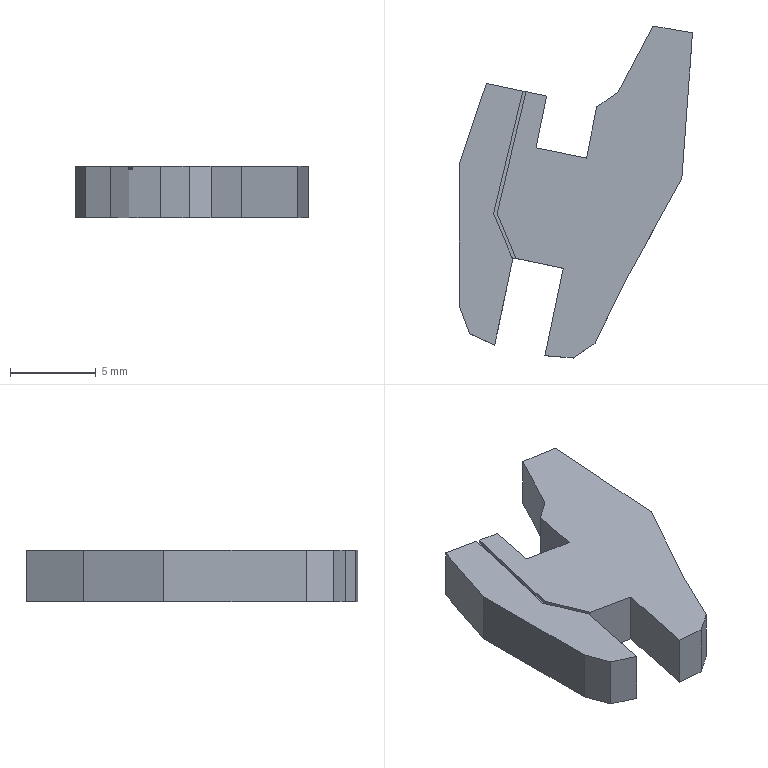Part | SolidWorks | features BaseBody 1 | 1 solid | 27 faces | box 13.603 x 19.375 x 3 mm | volume 451.595 mm3 | plane 15 | spline 12
STEP:
#1=CARTESIAN_POINT('',(66.198,112.5,1.3));
#2=VERTEX_POINT('',#1);
#3=CARTESIAN_POINT('',(66.394,112.459,1.3));
#4=VERTEX_POINT('',#3);
#5=CARTESIAN_POINT('',(66.198,112.5,1.3));
#6=CARTESIAN_POINT('',(66.263,112.486,1.3));
#7=CARTESIAN_POINT('',(66.329,112.473,1.3));
#8=CARTESIAN_POINT('',(66.394,112.459,1.3));
#9=B_SPLINE_CURVE_WITH_KNOTS('',3,(#5,#6,#7,#8),.UNSPECIFIED.,.F.,.F.,(4,4),(0.4488,0.4503),.UNSPECIFIED.);
#10=EDGE_CURVE('',#2,#4,#9,.T.);
#11=ORIENTED_EDGE('',*,*,#10,.F.);
#12=CARTESIAN_POINT('',(64.493,105.356,1.3));
#13=VERTEX_POINT('',#12);
#14=CARTESIAN_POINT('',(66.589,114.138,1.3));
#15=DIRECTION('',(-0.2321,-0.9727,0.));
#16=VECTOR('',#15,1000.);
#17=LINE('',#14,#16);
#18=EDGE_CURVE('',#2,#13,#17,.T.);
#19=ORIENTED_EDGE('',*,*,#18,.T.);
#20=CARTESIAN_POINT('',(65.611,102.69,1.3));
#21=VERTEX_POINT('',#20);
#22=CARTESIAN_POINT('',(64.493,105.356,1.3));
#23=DIRECTION('',(0.3866,-0.9222,0.));
#24=VECTOR('',#23,1000.);
#25=LINE('',#22,#24);
#26=EDGE_CURVE('',#13,#21,#25,.T.);
#27=ORIENTED_EDGE('',*,*,#26,.T.);
#28=CARTESIAN_POINT('',(65.627,102.768,1.3));
#29=VERTEX_POINT('',#28);
#30=CARTESIAN_POINT('',(42.225,-8.853,1.3));
#31=DIRECTION('',(0.2052,0.9787,0.));
#32=VECTOR('',#31,1000.);
#33=LINE('',#30,#32);
#34=EDGE_CURVE('',#21,#29,#33,.T.);
#35=ORIENTED_EDGE('',*,*,#34,.T.);
#36=CARTESIAN_POINT('',(65.811,102.729,1.3));
#37=VERTEX_POINT('',#36);
#38=CARTESIAN_POINT('',(23.402,111.621,1.3));
#39=DIRECTION('',(-0.9787,0.2052,0.));
#40=VECTOR('',#39,1000.);
#41=LINE('',#38,#40);
#42=EDGE_CURVE('',#37,#29,#41,.T.);
#43=ORIENTED_EDGE('',*,*,#42,.F.);
#44=CARTESIAN_POINT('',(64.703,105.373,1.3));
#45=VERTEX_POINT('',#44);
#46=CARTESIAN_POINT('',(64.678,105.433,1.3));
#47=DIRECTION('',(0.3866,-0.9222,0.));
#48=VECTOR('',#47,1000.);
#49=LINE('',#46,#48);
#50=EDGE_CURVE('',#45,#37,#49,.T.);
#51=ORIENTED_EDGE('',*,*,#50,.F.);
#52=CARTESIAN_POINT('',(66.784,114.092,1.3));
#53=DIRECTION('',(-0.2321,-0.9727,0.));
#54=VECTOR('',#53,1000.);
#55=LINE('',#52,#54);
#56=EDGE_CURVE('',#4,#45,#55,.T.);
#57=ORIENTED_EDGE('',*,*,#56,.F.);
#58=EDGE_LOOP('',(#11,#19,#27,#35,#43,#51,#57));
#59=FACE_OUTER_BOUND('',#58,.T.);
#60=CARTESIAN_POINT('',(0.,0.,1.3));
#61=DIRECTION('',(0.,0.,-1.));
#62=DIRECTION('',(0.,-1.,0.));
#63=AXIS2_PLACEMENT_3D('',#60,#61,#62);
#64=PLANE('',#63);
#65=ADVANCED_FACE('',(#59),#64,.F.);
#66=ORIENTED_EDGE('',*,*,#18,.F.);
#67=CARTESIAN_POINT('',(66.198,112.5,1.5));
#68=VERTEX_POINT('',#67);
#69=CARTESIAN_POINT('',(66.198,112.5,1.5));
#70=DIRECTION('',(0.,0.,1.));
#71=VECTOR('',#70,1000.);
#72=LINE('',#69,#71);
#73=EDGE_CURVE('',#2,#68,#72,.T.);
#74=ORIENTED_EDGE('',*,*,#73,.T.);
#75=CARTESIAN_POINT('',(64.493,105.356,1.5));
#76=VERTEX_POINT('',#75);
#77=CARTESIAN_POINT('',(37.228,-8.885,1.5));
#78=DIRECTION('',(-0.2321,-0.9727,0.));
#79=VECTOR('',#78,1000.);
#80=LINE('',#77,#79);
#81=EDGE_CURVE('',#68,#76,#80,.T.);
#82=ORIENTED_EDGE('',*,*,#81,.T.);
#83=CARTESIAN_POINT('',(64.493,105.356,1.3));
#84=DIRECTION('',(0.,0.,1.));
#85=VECTOR('',#84,1000.);
#86=LINE('',#83,#85);
#87=EDGE_CURVE('',#13,#76,#86,.T.);
#88=ORIENTED_EDGE('',*,*,#87,.F.);
#89=EDGE_LOOP('',(#66,#74,#82,#88));
#90=FACE_OUTER_BOUND('',#89,.T.);
#91=CARTESIAN_POINT('',(66.589,114.138,1.3));
#92=DIRECTION('',(0.9727,-0.2321,0.));
#93=DIRECTION('',(0.,0.,-1.));
#94=AXIS2_PLACEMENT_3D('',#91,#92,#93);
#95=PLANE('',#94);
#96=ADVANCED_FACE('',(#90),#95,.T.);
#97=CARTESIAN_POINT('',(66.394,112.459,1.5));
#98=VERTEX_POINT('',#97);
#99=CARTESIAN_POINT('',(66.394,112.459,1.5));
#100=DIRECTION('',(0.,0.,1.));
#101=VECTOR('',#100,1000.);
#102=LINE('',#99,#101);
#103=EDGE_CURVE('',#4,#98,#102,.T.);
#104=ORIENTED_EDGE('',*,*,#103,.F.);
#105=ORIENTED_EDGE('',*,*,#56,.T.);
#106=CARTESIAN_POINT('',(64.703,105.373,1.5));
#107=VERTEX_POINT('',#106);
#108=CARTESIAN_POINT('',(64.703,105.373,1.3));
#109=DIRECTION('',(0.,0.,1.));
#110=VECTOR('',#109,1000.);
#111=LINE('',#108,#110);
#112=EDGE_CURVE('',#45,#107,#111,.T.);
#113=ORIENTED_EDGE('',*,*,#112,.T.);
#114=CARTESIAN_POINT('',(37.423,-8.931,1.5));
#115=DIRECTION('',(-0.2321,-0.9727,0.));
#116=VECTOR('',#115,1000.);
#117=LINE('',#114,#116);
#118=EDGE_CURVE('',#98,#107,#117,.T.);
#119=ORIENTED_EDGE('',*,*,#118,.F.);
#120=EDGE_LOOP('',(#104,#105,#113,#119));
#121=FACE_OUTER_BOUND('',#120,.T.);
#122=CARTESIAN_POINT('',(66.784,114.092,1.3));
#123=DIRECTION('',(0.9727,-0.2321,0.));
#124=DIRECTION('',(0.,0.,-1.));
#125=AXIS2_PLACEMENT_3D('',#122,#123,#124);
#126=PLANE('',#125);
#127=ADVANCED_FACE('',(#121),#126,.F.);
#128=CARTESIAN_POINT('',(65.811,102.729,1.5));
#129=VERTEX_POINT('',#128);
#130=CARTESIAN_POINT('',(65.811,102.729,1.5));
#131=DIRECTION('',(0.,0.,-1.));
#132=VECTOR('',#131,1000.);
#133=LINE('',#130,#132);
#134=EDGE_CURVE('',#129,#37,#133,.T.);
#135=ORIENTED_EDGE('',*,*,#134,.F.);
#136=CARTESIAN_POINT('',(64.678,105.433,1.5));
#137=DIRECTION('',(0.3866,-0.9222,0.));
#138=VECTOR('',#137,1000.);
#139=LINE('',#136,#138);
#140=EDGE_CURVE('',#107,#129,#139,.T.);
#141=ORIENTED_EDGE('',*,*,#140,.F.);
#142=ORIENTED_EDGE('',*,*,#112,.F.);
#143=ORIENTED_EDGE('',*,*,#50,.T.);
#144=EDGE_LOOP('',(#135,#141,#142,#143));
#145=FACE_OUTER_BOUND('',#144,.T.);
#146=CARTESIAN_POINT('',(64.678,105.433,1.3));
#147=DIRECTION('',(0.9222,0.3866,0.));
#148=DIRECTION('',(0.,0.,-1.));
#149=AXIS2_PLACEMENT_3D('',#146,#147,#148);
#150=PLANE('',#149);
#151=ADVANCED_FACE('',(#145),#150,.F.);
#152=CARTESIAN_POINT('',(65.611,102.69,1.5));
#153=VERTEX_POINT('',#152);
#154=CARTESIAN_POINT('',(65.611,102.69,1.5));
#155=DIRECTION('',(0.,0.,1.));
#156=VECTOR('',#155,1000.);
#157=LINE('',#154,#156);
#158=EDGE_CURVE('',#21,#153,#157,.T.);
#159=ORIENTED_EDGE('',*,*,#158,.F.);
#160=ORIENTED_EDGE('',*,*,#26,.F.);
#161=ORIENTED_EDGE('',*,*,#87,.T.);
#162=CARTESIAN_POINT('',(64.493,105.356,1.5));
#163=DIRECTION('',(0.3866,-0.9222,0.));
#164=VECTOR('',#163,1000.);
#165=LINE('',#162,#164);
#166=EDGE_CURVE('',#76,#153,#165,.T.);
#167=ORIENTED_EDGE('',*,*,#166,.T.);
#168=EDGE_LOOP('',(#159,#160,#161,#167));
#169=FACE_OUTER_BOUND('',#168,.T.);
#170=CARTESIAN_POINT('',(64.493,105.356,1.3));
#171=DIRECTION('',(0.9222,0.3866,0.));
#172=DIRECTION('',(0.,0.,-1.));
#173=AXIS2_PLACEMENT_3D('',#170,#171,#172);
#174=PLANE('',#173);
#175=ADVANCED_FACE('',(#169),#174,.T.);
#176=CARTESIAN_POINT('',(64.074,112.946,-1.5));
#177=VERTEX_POINT('',#176);
#178=CARTESIAN_POINT('',(62.506,108.263,-1.5));
#179=VERTEX_POINT('',#178);
#180=CARTESIAN_POINT('',(64.074,112.946,-1.5));
#181=CARTESIAN_POINT('',(63.551,111.385,-1.5));
#182=CARTESIAN_POINT('',(63.029,109.824,-1.5));
#183=CARTESIAN_POINT('',(62.506,108.263,-1.5));
#184=B_SPLINE_CURVE_WITH_KNOTS('',3,(#180,#181,#182,#183),.UNSPECIFIED.,.F.,.F.,(4,4),(0.4595,0.4865),.UNSPECIFIED.);
#185=EDGE_CURVE('',#177,#179,#184,.T.);
#186=ORIENTED_EDGE('',*,*,#185,.F.);
#187=CARTESIAN_POINT('',(67.59,112.208,-1.5));
#188=VERTEX_POINT('',#187);
#189=CARTESIAN_POINT('',(67.59,112.208,-1.5));
#190=CARTESIAN_POINT('',(66.416,112.454,-1.5));
#191=CARTESIAN_POINT('',(65.247,112.7,-1.5));
#192=CARTESIAN_POINT('',(64.074,112.946,-1.5));
#193=B_SPLINE_CURVE_WITH_KNOTS('',3,(#189,#190,#191,#192),.UNSPECIFIED.,.F.,.F.,(4,4),(0.4324,0.4595),.UNSPECIFIED.);
#194=EDGE_CURVE('',#188,#177,#193,.T.);
#195=ORIENTED_EDGE('',*,*,#194,.F.);
#196=CARTESIAN_POINT('',(66.974,109.185,-1.5));
#197=VERTEX_POINT('',#196);
#198=CARTESIAN_POINT('',(42.966,-8.747,-1.5));
#199=DIRECTION('',(-0.1995,-0.9799,0.));
#200=VECTOR('',#199,1000.);
#201=LINE('',#198,#200);
#202=EDGE_CURVE('',#188,#197,#201,.T.);
#203=ORIENTED_EDGE('',*,*,#202,.T.);
#204=CARTESIAN_POINT('',(69.914,108.586,-1.5));
#205=VERTEX_POINT('',#204);
#206=CARTESIAN_POINT('',(24.008,117.932,-1.5));
#207=DIRECTION('',(0.9799,-0.1995,0.));
#208=VECTOR('',#207,1000.);
#209=LINE('',#206,#208);
#210=EDGE_CURVE('',#197,#205,#209,.T.);
#211=ORIENTED_EDGE('',*,*,#210,.T.);
#212=CARTESIAN_POINT('',(70.523,111.576,-1.5));
#213=VERTEX_POINT('',#212);
#214=CARTESIAN_POINT('',(45.905,-9.345,-1.5));
#215=DIRECTION('',(-0.1995,-0.9799,0.));
#216=VECTOR('',#215,1000.);
#217=LINE('',#214,#216);
#218=EDGE_CURVE('',#213,#205,#217,.T.);
#219=ORIENTED_EDGE('',*,*,#218,.F.);
#220=CARTESIAN_POINT('',(71.782,112.463,-1.5));
#221=VERTEX_POINT('',#220);
#222=CARTESIAN_POINT('',(71.782,112.463,-1.5));
#223=CARTESIAN_POINT('',(71.368,112.172,-1.5));
#224=CARTESIAN_POINT('',(70.946,111.878,-1.5));
#225=CARTESIAN_POINT('',(70.529,111.581,-1.5));
#226=CARTESIAN_POINT('',(70.523,111.576,-1.5));
#227=B_SPLINE_CURVE_WITH_KNOTS('',3,(#222,#223,#224,#225,#226),.UNSPECIFIED.,.F.,.F.,(4,1,4),(0.3243,0.3514,0.3518),.UNSPECIFIED.);
#228=EDGE_CURVE('',#221,#213,#227,.T.);
#229=ORIENTED_EDGE('',*,*,#228,.F.);
#230=CARTESIAN_POINT('',(73.791,116.299,-1.5));
#231=VERTEX_POINT('',#230);
#232=CARTESIAN_POINT('',(73.791,116.299,-1.5));
#233=CARTESIAN_POINT('',(73.122,115.02,-1.5));
#234=CARTESIAN_POINT('',(72.451,113.741,-1.5));
#235=CARTESIAN_POINT('',(71.782,112.463,-1.5));
#236=B_SPLINE_CURVE_WITH_KNOTS('',3,(#232,#233,#234,#235),.UNSPECIFIED.,.F.,.F.,(4,4),(0.2973,0.3243),.UNSPECIFIED.);
#237=EDGE_CURVE('',#231,#221,#236,.T.);
#238=ORIENTED_EDGE('',*,*,#237,.F.);
#239=CARTESIAN_POINT('',(76.109,115.9,-1.5));
#240=VERTEX_POINT('',#239);
#241=CARTESIAN_POINT('',(76.109,115.9,-1.5));
#242=CARTESIAN_POINT('',(75.336,116.034,-1.5));
#243=CARTESIAN_POINT('',(74.563,116.165,-1.5));
#244=CARTESIAN_POINT('',(73.791,116.299,-1.5));
#245=B_SPLINE_CURVE_WITH_KNOTS('',3,(#241,#242,#243,#244),.UNSPECIFIED.,.F.,.F.,(4,4),(0.2703,0.2973),.UNSPECIFIED.);
#246=EDGE_CURVE('',#240,#231,#245,.T.);
#247=ORIENTED_EDGE('',*,*,#246,.F.);
#248=CARTESIAN_POINT('',(75.486,107.399,-1.5));
#249=VERTEX_POINT('',#248);
#250=CARTESIAN_POINT('',(75.486,107.399,-1.5));
#251=CARTESIAN_POINT('',(75.695,110.235,-1.5));
#252=CARTESIAN_POINT('',(75.9,113.068,-1.5));
#253=CARTESIAN_POINT('',(76.109,115.9,-1.5));
#254=B_SPLINE_CURVE_WITH_KNOTS('',3,(#250,#251,#252,#253),.UNSPECIFIED.,.F.,.F.,(4,4),(0.2432,0.2703),.UNSPECIFIED.);
#255=EDGE_CURVE('',#249,#240,#254,.T.);
#256=ORIENTED_EDGE('',*,*,#255,.F.);
#257=CARTESIAN_POINT('',(72.174,101.392,-1.5));
#258=VERTEX_POINT('',#257);
#259=CARTESIAN_POINT('',(72.174,101.392,-1.5));
#260=CARTESIAN_POINT('',(73.277,103.395,-1.5));
#261=CARTESIAN_POINT('',(74.383,105.398,-1.5));
#262=CARTESIAN_POINT('',(75.486,107.399,-1.5));
#263=B_SPLINE_CURVE_WITH_KNOTS('',3,(#259,#260,#261,#262),.UNSPECIFIED.,.F.,.F.,(4,4),(0.2162,0.2432),.UNSPECIFIED.);
#264=EDGE_CURVE('',#258,#249,#263,.T.);
#265=ORIENTED_EDGE('',*,*,#264,.F.);
#266=CARTESIAN_POINT('',(70.417,97.774,-1.5));
#267=VERTEX_POINT('',#266);
#268=CARTESIAN_POINT('',(70.417,97.774,-1.5));
#269=CARTESIAN_POINT('',(71.002,98.978,-1.5));
#270=CARTESIAN_POINT('',(71.586,100.184,-1.5));
#271=CARTESIAN_POINT('',(72.174,101.392,-1.5));
#272=B_SPLINE_CURVE_WITH_KNOTS('',3,(#268,#269,#270,#271),.UNSPECIFIED.,.F.,.F.,(4,4),(0.1892,0.2162),.UNSPECIFIED.);
#273=EDGE_CURVE('',#267,#258,#272,.T.);
#274=ORIENTED_EDGE('',*,*,#273,.F.);
#275=CARTESIAN_POINT('',(69.133,96.923,-1.5));
#276=VERTEX_POINT('',#275);
#277=CARTESIAN_POINT('',(69.133,96.923,-1.5));
#278=CARTESIAN_POINT('',(69.561,97.206,-1.5));
#279=CARTESIAN_POINT('',(69.989,97.49,-1.5));
#280=CARTESIAN_POINT('',(70.417,97.774,-1.5));
#281=B_SPLINE_CURVE_WITH_KNOTS('',3,(#277,#278,#279,#280),.UNSPECIFIED.,.F.,.F.,(4,4),(0.1622,0.1892),.UNSPECIFIED.);
#282=EDGE_CURVE('',#276,#267,#281,.T.);
#283=ORIENTED_EDGE('',*,*,#282,.F.);
#284=CARTESIAN_POINT('',(67.494,97.055,-1.5));
#285=VERTEX_POINT('',#284);
#286=CARTESIAN_POINT('',(67.494,97.055,-1.5));
#287=CARTESIAN_POINT('',(68.041,97.01,-1.5));
#288=CARTESIAN_POINT('',(68.588,96.967,-1.5));
#289=CARTESIAN_POINT('',(69.133,96.923,-1.5));
#290=B_SPLINE_CURVE_WITH_KNOTS('',3,(#286,#287,#288,#289),.UNSPECIFIED.,.F.,.F.,(4,4),(0.1351,0.1622),.UNSPECIFIED.);
#291=EDGE_CURVE('',#285,#276,#290,.T.);
#292=ORIENTED_EDGE('',*,*,#291,.F.);
#293=CARTESIAN_POINT('',(68.563,102.152,-1.5));
#294=VERTEX_POINT('',#293);
#295=CARTESIAN_POINT('',(45.161,-9.468,-1.5));
#296=DIRECTION('',(-0.2052,-0.9787,0.));
#297=VECTOR('',#296,1000.);
#298=LINE('',#295,#297);
#299=EDGE_CURVE('',#294,#285,#298,.T.);
#300=ORIENTED_EDGE('',*,*,#299,.F.);
#301=CARTESIAN_POINT('',(65.627,102.768,-1.5));
#302=VERTEX_POINT('',#301);
#303=CARTESIAN_POINT('',(23.402,111.621,-1.5));
#304=DIRECTION('',(0.9787,-0.2052,0.));
#305=VECTOR('',#304,1000.);
#306=LINE('',#303,#305);
#307=EDGE_CURVE('',#302,#294,#306,.T.);
#308=ORIENTED_EDGE('',*,*,#307,.F.);
#309=CARTESIAN_POINT('',(64.558,97.671,-1.5));
#310=VERTEX_POINT('',#309);
#311=CARTESIAN_POINT('',(42.225,-8.853,-1.5));
#312=DIRECTION('',(-0.2052,-0.9787,0.));
#313=VECTOR('',#312,1000.);
#314=LINE('',#311,#313);
#315=EDGE_CURVE('',#302,#310,#314,.T.);
#316=ORIENTED_EDGE('',*,*,#315,.T.);
#317=CARTESIAN_POINT('',(63.093,98.343,-1.5));
#318=VERTEX_POINT('',#317);
#319=CARTESIAN_POINT('',(63.093,98.343,-1.5));
#320=CARTESIAN_POINT('',(63.582,98.12,-1.5));
#321=CARTESIAN_POINT('',(64.069,97.895,-1.5));
#322=CARTESIAN_POINT('',(64.558,97.671,-1.5));
#323=B_SPLINE_CURVE_WITH_KNOTS('',3,(#319,#320,#321,#322),.UNSPECIFIED.,.F.,.F.,(4,4),(0.02703,0.05397),.UNSPECIFIED.);
#324=EDGE_CURVE('',#318,#310,#323,.T.);
#325=ORIENTED_EDGE('',*,*,#324,.F.);
#326=CARTESIAN_POINT('',(62.506,99.936,-1.5));
#327=VERTEX_POINT('',#326);
#328=CARTESIAN_POINT('',(62.506,99.936,-1.5));
#329=CARTESIAN_POINT('',(62.702,99.405,-1.5));
#330=CARTESIAN_POINT('',(62.897,98.875,-1.5));
#331=CARTESIAN_POINT('',(63.093,98.343,-1.5));
#332=B_SPLINE_CURVE_WITH_KNOTS('',3,(#328,#329,#330,#331),.UNSPECIFIED.,.F.,.F.,(4,4),(0.,0.02703),.UNSPECIFIED.);
#333=EDGE_CURVE('',#327,#318,#332,.T.);
#334=ORIENTED_EDGE('',*,*,#333,.F.);
#335=CARTESIAN_POINT('',(62.506,0.,-1.5));
#336=DIRECTION('',(0.,-1.,0.));
#337=VECTOR('',#336,1000.);
#338=LINE('',#335,#337);
#339=EDGE_CURVE('',#179,#327,#338,.T.);
#340=ORIENTED_EDGE('',*,*,#339,.F.);
#341=EDGE_LOOP('',(#186,#195,#203,#211,#219,#229,#238,#247,#256,#265,#274,#283,#292,#300,#308,#316,#325,#334,#340));
#342=FACE_OUTER_BOUND('',#341,.T.);
#343=CARTESIAN_POINT('',(0.,0.,-1.5));
#344=DIRECTION('',(0.,0.,1.));
#345=DIRECTION('',(1.,0.,0.));
#346=AXIS2_PLACEMENT_3D('',#343,#344,#345);
#347=PLANE('',#346);
#348=ADVANCED_FACE('',(#342),#347,.F.);
#349=ORIENTED_EDGE('',*,*,#140,.T.);
#350=CARTESIAN_POINT('',(68.563,102.152,1.5));
#351=VERTEX_POINT('',#350);
#352=CARTESIAN_POINT('',(23.402,111.621,1.5));
#353=DIRECTION('',(0.9787,-0.2052,0.));
#354=VECTOR('',#353,1000.);
#355=LINE('',#352,#354);
#356=EDGE_CURVE('',#129,#351,#355,.T.);
#357=ORIENTED_EDGE('',*,*,#356,.T.);
#358=CARTESIAN_POINT('',(67.494,97.055,1.5));
#359=VERTEX_POINT('',#358);
#360=CARTESIAN_POINT('',(45.161,-9.468,1.5));
#361=DIRECTION('',(-0.2052,-0.9787,0.));
#362=VECTOR('',#361,1000.);
#363=LINE('',#360,#362);
#364=EDGE_CURVE('',#351,#359,#363,.T.);
#365=ORIENTED_EDGE('',*,*,#364,.T.);
#366=CARTESIAN_POINT('',(69.133,96.923,1.5));
#367=VERTEX_POINT('',#366);
#368=CARTESIAN_POINT('',(67.494,97.055,1.5));
#369=CARTESIAN_POINT('',(68.041,97.01,1.5));
#370=CARTESIAN_POINT('',(68.588,96.967,1.5));
#371=CARTESIAN_POINT('',(69.133,96.923,1.5));
#372=B_SPLINE_CURVE_WITH_KNOTS('',3,(#368,#369,#370,#371),.UNSPECIFIED.,.F.,.F.,(4,4),(0.1351,0.1622),.UNSPECIFIED.);
#373=EDGE_CURVE('',#359,#367,#372,.T.);
#374=ORIENTED_EDGE('',*,*,#373,.T.);
#375=CARTESIAN_POINT('',(70.417,97.774,1.5));
#376=VERTEX_POINT('',#375);
#377=CARTESIAN_POINT('',(69.133,96.923,1.5));
#378=CARTESIAN_POINT('',(69.561,97.206,1.5));
#379=CARTESIAN_POINT('',(69.989,97.49,1.5));
#380=CARTESIAN_POINT('',(70.417,97.774,1.5));
#381=B_SPLINE_CURVE_WITH_KNOTS('',3,(#377,#378,#379,#380),.UNSPECIFIED.,.F.,.F.,(4,4),(0.1622,0.1892),.UNSPECIFIED.);
#382=EDGE_CURVE('',#367,#376,#381,.T.);
#383=ORIENTED_EDGE('',*,*,#382,.T.);
#384=CARTESIAN_POINT('',(72.174,101.392,1.5));
#385=VERTEX_POINT('',#384);
#386=CARTESIAN_POINT('',(70.417,97.774,1.5));
#387=CARTESIAN_POINT('',(71.002,98.978,1.5));
#388=CARTESIAN_POINT('',(71.586,100.184,1.5));
#389=CARTESIAN_POINT('',(72.174,101.392,1.5));
#390=B_SPLINE_CURVE_WITH_KNOTS('',3,(#386,#387,#388,#389),.UNSPECIFIED.,.F.,.F.,(4,4),(0.1892,0.2162),.UNSPECIFIED.);
#391=EDGE_CURVE('',#376,#385,#390,.T.);
#392=ORIENTED_EDGE('',*,*,#391,.T.);
#393=CARTESIAN_POINT('',(75.486,107.399,1.5));
#394=VERTEX_POINT('',#393);
#395=CARTESIAN_POINT('',(72.174,101.392,1.5));
#396=CARTESIAN_POINT('',(73.277,103.395,1.5));
#397=CARTESIAN_POINT('',(74.383,105.398,1.5));
#398=CARTESIAN_POINT('',(75.486,107.399,1.5));
#399=B_SPLINE_CURVE_WITH_KNOTS('',3,(#395,#396,#397,#398),.UNSPECIFIED.,.F.,.F.,(4,4),(0.2162,0.2432),.UNSPECIFIED.);
#400=EDGE_CURVE('',#385,#394,#399,.T.);
#401=ORIENTED_EDGE('',*,*,#400,.T.);
#402=CARTESIAN_POINT('',(76.109,115.9,1.5));
#403=VERTEX_POINT('',#402);
#404=CARTESIAN_POINT('',(75.486,107.399,1.5));
#405=CARTESIAN_POINT('',(75.695,110.235,1.5));
#406=CARTESIAN_POINT('',(75.9,113.068,1.5));
#407=CARTESIAN_POINT('',(76.109,115.9,1.5));
#408=B_SPLINE_CURVE_WITH_KNOTS('',3,(#404,#405,#406,#407),.UNSPECIFIED.,.F.,.F.,(4,4),(0.2432,0.2703),.UNSPECIFIED.);
#409=EDGE_CURVE('',#394,#403,#408,.T.);
#410=ORIENTED_EDGE('',*,*,#409,.T.);
#411=CARTESIAN_POINT('',(73.791,116.299,1.5));
#412=VERTEX_POINT('',#411);
#413=CARTESIAN_POINT('',(76.109,115.9,1.5));
#414=CARTESIAN_POINT('',(75.336,116.034,1.5));
#415=CARTESIAN_POINT('',(74.563,116.165,1.5));
#416=CARTESIAN_POINT('',(73.791,116.299,1.5));
#417=B_SPLINE_CURVE_WITH_KNOTS('',3,(#413,#414,#415,#416),.UNSPECIFIED.,.F.,.F.,(4,4),(0.2703,0.2973),.UNSPECIFIED.);
#418=EDGE_CURVE('',#403,#412,#417,.T.);
#419=ORIENTED_EDGE('',*,*,#418,.T.);
#420=CARTESIAN_POINT('',(71.782,112.463,1.5));
#421=VERTEX_POINT('',#420);
#422=CARTESIAN_POINT('',(73.791,116.299,1.5));
#423=CARTESIAN_POINT('',(73.122,115.02,1.5));
#424=CARTESIAN_POINT('',(72.451,113.741,1.5));
#425=CARTESIAN_POINT('',(71.782,112.463,1.5));
#426=B_SPLINE_CURVE_WITH_KNOTS('',3,(#422,#423,#424,#425),.UNSPECIFIED.,.F.,.F.,(4,4),(0.2973,0.3243),.UNSPECIFIED.);
#427=EDGE_CURVE('',#412,#421,#426,.T.);
#428=ORIENTED_EDGE('',*,*,#427,.T.);
#429=CARTESIAN_POINT('',(70.523,111.576,1.5));
#430=VERTEX_POINT('',#429);
#431=CARTESIAN_POINT('',(71.782,112.463,1.5));
#432=CARTESIAN_POINT('',(71.368,112.172,1.5));
#433=CARTESIAN_POINT('',(70.946,111.878,1.5));
#434=CARTESIAN_POINT('',(70.529,111.581,1.5));
#435=CARTESIAN_POINT('',(70.523,111.576,1.5));
#436=B_SPLINE_CURVE_WITH_KNOTS('',3,(#431,#432,#433,#434,#435),.UNSPECIFIED.,.F.,.F.,(4,1,4),(0.3243,0.3514,0.3518),.UNSPECIFIED.);
#437=EDGE_CURVE('',#421,#430,#436,.T.);
#438=ORIENTED_EDGE('',*,*,#437,.T.);
#439=CARTESIAN_POINT('',(69.914,108.586,1.5));
#440=VERTEX_POINT('',#439);
#441=CARTESIAN_POINT('',(45.905,-9.345,1.5));
#442=DIRECTION('',(-0.1995,-0.9799,0.));
#443=VECTOR('',#442,1000.);
#444=LINE('',#441,#443);
#445=EDGE_CURVE('',#430,#440,#444,.T.);
#446=ORIENTED_EDGE('',*,*,#445,.T.);
#447=CARTESIAN_POINT('',(66.974,109.185,1.5));
#448=VERTEX_POINT('',#447);
#449=CARTESIAN_POINT('',(24.008,117.932,1.5));
#450=DIRECTION('',(0.9799,-0.1995,0.));
#451=VECTOR('',#450,1000.);
#452=LINE('',#449,#451);
#453=EDGE_CURVE('',#448,#440,#452,.T.);
#454=ORIENTED_EDGE('',*,*,#453,.F.);
#455=CARTESIAN_POINT('',(67.59,112.208,1.5));
#456=VERTEX_POINT('',#455);
#457=CARTESIAN_POINT('',(42.966,-8.747,1.5));
#458=DIRECTION('',(-0.1995,-0.9799,0.));
#459=VECTOR('',#458,1000.);
#460=LINE('',#457,#459);
#461=EDGE_CURVE('',#456,#448,#460,.T.);
#462=ORIENTED_EDGE('',*,*,#461,.F.);
#463=CARTESIAN_POINT('',(67.59,112.208,1.5));
#464=CARTESIAN_POINT('',(67.191,112.292,1.5));
#465=CARTESIAN_POINT('',(66.792,112.375,1.5));
#466=CARTESIAN_POINT('',(66.394,112.459,1.5));
#467=B_SPLINE_CURVE_WITH_KNOTS('',3,(#463,#464,#465,#466),.UNSPECIFIED.,.F.,.F.,(4,4),(0.4324,0.4416),.UNSPECIFIED.);
#468=EDGE_CURVE('',#456,#98,#467,.T.);
#469=ORIENTED_EDGE('',*,*,#468,.T.);
#470=ORIENTED_EDGE('',*,*,#118,.T.);
#471=EDGE_LOOP('',(#349,#357,#365,#374,#383,#392,#401,#410,#419,#428,#438,#446,#454,#462,#469,#470));
#472=FACE_OUTER_BOUND('',#471,.T.);
#473=CARTESIAN_POINT('',(0.,0.,1.5));
#474=DIRECTION('',(0.,0.,1.));
#475=DIRECTION('',(1.,0.,0.));
#476=AXIS2_PLACEMENT_3D('',#473,#474,#475);
#477=PLANE('',#476);
#478=ADVANCED_FACE('',(#472),#477,.T.);
#479=ORIENTED_EDGE('',*,*,#339,.T.);
#480=CARTESIAN_POINT('',(62.506,99.936,1.5));
#481=VERTEX_POINT('',#480);
#482=CARTESIAN_POINT('',(62.506,99.936,1.5));
#483=DIRECTION('',(0.,0.,-1.));
#484=VECTOR('',#483,1000.);
#485=LINE('',#482,#484);
#486=EDGE_CURVE('',#481,#327,#485,.T.);
#487=ORIENTED_EDGE('',*,*,#486,.F.);
#488=CARTESIAN_POINT('',(62.506,108.263,1.5));
#489=VERTEX_POINT('',#488);
#490=CARTESIAN_POINT('',(62.506,0.,1.5));
#491=DIRECTION('',(0.,-1.,0.));
#492=VECTOR('',#491,1000.);
#493=LINE('',#490,#492);
#494=EDGE_CURVE('',#489,#481,#493,.T.);
#495=ORIENTED_EDGE('',*,*,#494,.F.);
#496=CARTESIAN_POINT('',(62.506,108.263,1.5));
#497=DIRECTION('',(0.,0.,-1.));
#498=VECTOR('',#497,1000.);
#499=LINE('',#496,#498);
#500=EDGE_CURVE('',#489,#179,#499,.T.);
#501=ORIENTED_EDGE('',*,*,#500,.T.);
#502=EDGE_LOOP('',(#479,#487,#495,#501));
#503=FACE_OUTER_BOUND('',#502,.T.);
#504=CARTESIAN_POINT('',(62.506,0.,1.5));
#505=DIRECTION('',(-1.,0.,0.));
#506=DIRECTION('',(0.,0.,1.));
#507=AXIS2_PLACEMENT_3D('',#504,#505,#506);
#508=PLANE('',#507);
#509=ADVANCED_FACE('',(#503),#508,.T.);
#510=ORIENTED_EDGE('',*,*,#333,.T.);
#511=CARTESIAN_POINT('',(63.093,98.343,1.5));
#512=VERTEX_POINT('',#511);
#513=CARTESIAN_POINT('',(63.093,98.343,1.5));
#514=DIRECTION('',(0.,0.,-1.));
#515=VECTOR('',#514,1000.);
#516=LINE('',#513,#515);
#517=EDGE_CURVE('',#512,#318,#516,.T.);
#518=ORIENTED_EDGE('',*,*,#517,.F.);
#519=CARTESIAN_POINT('',(62.506,99.936,1.5));
#520=CARTESIAN_POINT('',(62.702,99.405,1.5));
#521=CARTESIAN_POINT('',(62.897,98.875,1.5));
#522=CARTESIAN_POINT('',(63.093,98.343,1.5));
#523=B_SPLINE_CURVE_WITH_KNOTS('',3,(#519,#520,#521,#522),.UNSPECIFIED.,.F.,.F.,(4,4),(0.,0.02703),.UNSPECIFIED.);
#524=EDGE_CURVE('',#481,#512,#523,.T.);
#525=ORIENTED_EDGE('',*,*,#524,.F.);
#526=ORIENTED_EDGE('',*,*,#486,.T.);
#527=EDGE_LOOP('',(#510,#518,#525,#526));
#528=FACE_OUTER_BOUND('',#527,.T.);
#529=CARTESIAN_POINT('',(63.093,98.343,1.5));
#530=CARTESIAN_POINT('',(63.093,98.343,-1.5));
#531=CARTESIAN_POINT('',(62.897,98.875,1.5));
#532=CARTESIAN_POINT('',(62.897,98.875,-1.5));
#533=CARTESIAN_POINT('',(62.702,99.405,1.5));
#534=CARTESIAN_POINT('',(62.702,99.405,-1.5));
#535=CARTESIAN_POINT('',(62.506,99.936,1.5));
#536=CARTESIAN_POINT('',(62.506,99.936,-1.5));
#537=B_SPLINE_SURFACE_WITH_KNOTS('',3,1,((#529,#530),(#531,#532),(#533,#534),(#535,#536)),.UNSPECIFIED.,.F.,.F.,.F.,(4,4),(2,2),(0.,0.02703),(0.,1.),.UNSPECIFIED.);
#538=ADVANCED_FACE('',(#528),#537,.T.);
#539=ORIENTED_EDGE('',*,*,#324,.T.);
#540=CARTESIAN_POINT('',(64.558,97.671,1.5));
#541=VERTEX_POINT('',#540);
#542=CARTESIAN_POINT('',(64.558,97.671,1.5));
#543=DIRECTION('',(0.,0.,-1.));
#544=VECTOR('',#543,1000.);
#545=LINE('',#542,#544);
#546=EDGE_CURVE('',#541,#310,#545,.T.);
#547=ORIENTED_EDGE('',*,*,#546,.F.);
#548=CARTESIAN_POINT('',(63.093,98.343,1.5));
#549=CARTESIAN_POINT('',(63.582,98.12,1.5));
#550=CARTESIAN_POINT('',(64.069,97.895,1.5));
#551=CARTESIAN_POINT('',(64.558,97.671,1.5));
#552=B_SPLINE_CURVE_WITH_KNOTS('',3,(#548,#549,#550,#551),.UNSPECIFIED.,.F.,.F.,(4,4),(0.02703,0.05397),.UNSPECIFIED.);
#553=EDGE_CURVE('',#512,#541,#552,.T.);
#554=ORIENTED_EDGE('',*,*,#553,.F.);
#555=ORIENTED_EDGE('',*,*,#517,.T.);
#556=EDGE_LOOP('',(#539,#547,#554,#555));
#557=FACE_OUTER_BOUND('',#556,.T.);
#558=CARTESIAN_POINT('',(64.558,97.671,1.5));
#559=CARTESIAN_POINT('',(64.558,97.671,-1.5));
#560=CARTESIAN_POINT('',(64.069,97.895,1.5));
#561=CARTESIAN_POINT('',(64.069,97.895,-1.5));
#562=CARTESIAN_POINT('',(63.582,98.12,1.5));
#563=CARTESIAN_POINT('',(63.582,98.12,-1.5));
#564=CARTESIAN_POINT('',(63.093,98.343,1.5));
#565=CARTESIAN_POINT('',(63.093,98.343,-1.5));
#566=B_SPLINE_SURFACE_WITH_KNOTS('',3,1,((#558,#559),(#560,#561),(#562,#563),(#564,#565)),.UNSPECIFIED.,.F.,.F.,.F.,(4,4),(2,2),(0.,0.02694),(0.,1.),.UNSPECIFIED.);
#567=ADVANCED_FACE('',(#557),#566,.T.);
#568=ORIENTED_EDGE('',*,*,#134,.T.);
#569=ORIENTED_EDGE('',*,*,#42,.T.);
#570=CARTESIAN_POINT('',(65.627,102.768,1.5));
#571=DIRECTION('',(0.,0.,-1.));
#572=VECTOR('',#571,1000.);
#573=LINE('',#570,#572);
#574=EDGE_CURVE('',#29,#302,#573,.T.);
#575=ORIENTED_EDGE('',*,*,#574,.T.);
#576=ORIENTED_EDGE('',*,*,#307,.T.);
#577=CARTESIAN_POINT('',(68.563,102.152,1.5));
#578=DIRECTION('',(0.,0.,-1.));
#579=VECTOR('',#578,1000.);
#580=LINE('',#577,#579);
#581=EDGE_CURVE('',#351,#294,#580,.T.);
#582=ORIENTED_EDGE('',*,*,#581,.F.);
#583=ORIENTED_EDGE('',*,*,#356,.F.);
#584=EDGE_LOOP('',(#568,#569,#575,#576,#582,#583));
#585=FACE_OUTER_BOUND('',#584,.T.);
#586=CARTESIAN_POINT('',(23.402,111.621,1.5));
#587=DIRECTION('',(-0.2052,-0.9787,0.));
#588=DIRECTION('',(-0.9787,0.2052,0.));
#589=AXIS2_PLACEMENT_3D('',#586,#587,#588);
#590=PLANE('',#589);
#591=ADVANCED_FACE('',(#585),#590,.T.);
#592=ORIENTED_EDGE('',*,*,#299,.T.);
#593=CARTESIAN_POINT('',(67.494,97.055,1.5));
#594=DIRECTION('',(0.,0.,-1.));
#595=VECTOR('',#594,1000.);
#596=LINE('',#593,#595);
#597=EDGE_CURVE('',#359,#285,#596,.T.);
#598=ORIENTED_EDGE('',*,*,#597,.F.);
#599=ORIENTED_EDGE('',*,*,#364,.F.);
#600=ORIENTED_EDGE('',*,*,#581,.T.);
#601=EDGE_LOOP('',(#592,#598,#599,#600));
#602=FACE_OUTER_BOUND('',#601,.T.);
#603=CARTESIAN_POINT('',(45.161,-9.468,1.5));
#604=DIRECTION('',(-0.9787,0.2052,0.));
#605=DIRECTION('',(0.,0.,1.));
#606=AXIS2_PLACEMENT_3D('',#603,#604,#605);
#607=PLANE('',#606);
#608=ADVANCED_FACE('',(#602),#607,.T.);
#609=ORIENTED_EDGE('',*,*,#291,.T.);
#610=CARTESIAN_POINT('',(69.133,96.923,1.5));
#611=DIRECTION('',(0.,0.,-1.));
#612=VECTOR('',#611,1000.);
#613=LINE('',#610,#612);
#614=EDGE_CURVE('',#367,#276,#613,.T.);
#615=ORIENTED_EDGE('',*,*,#614,.F.);
#616=ORIENTED_EDGE('',*,*,#373,.F.);
#617=ORIENTED_EDGE('',*,*,#597,.T.);
#618=EDGE_LOOP('',(#609,#615,#616,#617));
#619=FACE_OUTER_BOUND('',#618,.T.);
#620=CARTESIAN_POINT('',(69.133,96.923,1.5));
#621=CARTESIAN_POINT('',(69.133,96.923,-1.5));
#622=CARTESIAN_POINT('',(68.588,96.967,1.5));
#623=CARTESIAN_POINT('',(68.588,96.967,-1.5));
#624=CARTESIAN_POINT('',(68.041,97.01,1.5));
#625=CARTESIAN_POINT('',(68.041,97.01,-1.5));
#626=CARTESIAN_POINT('',(67.494,97.055,1.5));
#627=CARTESIAN_POINT('',(67.494,97.055,-1.5));
#628=B_SPLINE_SURFACE_WITH_KNOTS('',3,1,((#620,#621),(#622,#623),(#624,#625),(#626,#627)),.UNSPECIFIED.,.F.,.F.,.F.,(4,4),(2,2),(0.,0.02703),(0.,1.),.UNSPECIFIED.);
#629=ADVANCED_FACE('',(#619),#628,.T.);
#630=ORIENTED_EDGE('',*,*,#282,.T.);
#631=CARTESIAN_POINT('',(70.417,97.774,1.5));
#632=DIRECTION('',(0.,0.,-1.));
#633=VECTOR('',#632,1000.);
#634=LINE('',#631,#633);
#635=EDGE_CURVE('',#376,#267,#634,.T.);
#636=ORIENTED_EDGE('',*,*,#635,.F.);
#637=ORIENTED_EDGE('',*,*,#382,.F.);
#638=ORIENTED_EDGE('',*,*,#614,.T.);
#639=EDGE_LOOP('',(#630,#636,#637,#638));
#640=FACE_OUTER_BOUND('',#639,.T.);
#641=CARTESIAN_POINT('',(70.417,97.774,1.5));
#642=CARTESIAN_POINT('',(70.417,97.774,-1.5));
#643=CARTESIAN_POINT('',(69.989,97.49,1.5));
#644=CARTESIAN_POINT('',(69.989,97.49,-1.5));
#645=CARTESIAN_POINT('',(69.561,97.206,1.5));
#646=CARTESIAN_POINT('',(69.561,97.206,-1.5));
#647=CARTESIAN_POINT('',(69.133,96.923,1.5));
#648=CARTESIAN_POINT('',(69.133,96.923,-1.5));
#649=B_SPLINE_SURFACE_WITH_KNOTS('',3,1,((#641,#642),(#643,#644),(#645,#646),(#647,#648)),.UNSPECIFIED.,.F.,.F.,.F.,(4,4),(2,2),(0.,0.02703),(0.,1.),.UNSPECIFIED.);
#650=ADVANCED_FACE('',(#640),#649,.T.);
#651=ORIENTED_EDGE('',*,*,#273,.T.);
#652=CARTESIAN_POINT('',(72.174,101.392,1.5));
#653=DIRECTION('',(0.,0.,-1.));
#654=VECTOR('',#653,1000.);
#655=LINE('',#652,#654);
#656=EDGE_CURVE('',#385,#258,#655,.T.);
#657=ORIENTED_EDGE('',*,*,#656,.F.);
#658=ORIENTED_EDGE('',*,*,#391,.F.);
#659=ORIENTED_EDGE('',*,*,#635,.T.);
#660=EDGE_LOOP('',(#651,#657,#658,#659));
#661=FACE_OUTER_BOUND('',#660,.T.);
#662=CARTESIAN_POINT('',(72.174,101.392,1.5));
#663=CARTESIAN_POINT('',(72.174,101.392,-1.5));
#664=CARTESIAN_POINT('',(71.586,100.184,1.5));
#665=CARTESIAN_POINT('',(71.586,100.184,-1.5));
#666=CARTESIAN_POINT('',(71.002,98.978,1.5));
#667=CARTESIAN_POINT('',(71.002,98.978,-1.5));
#668=CARTESIAN_POINT('',(70.417,97.774,1.5));
#669=CARTESIAN_POINT('',(70.417,97.774,-1.5));
#670=B_SPLINE_SURFACE_WITH_KNOTS('',3,1,((#662,#663),(#664,#665),(#666,#667),(#668,#669)),.UNSPECIFIED.,.F.,.F.,.F.,(4,4),(2,2),(0.,0.02703),(0.,1.),.UNSPECIFIED.);
#671=ADVANCED_FACE('',(#661),#670,.T.);
#672=ORIENTED_EDGE('',*,*,#264,.T.);
#673=CARTESIAN_POINT('',(75.486,107.399,1.5));
#674=DIRECTION('',(0.,0.,-1.));
#675=VECTOR('',#674,1000.);
#676=LINE('',#673,#675);
#677=EDGE_CURVE('',#394,#249,#676,.T.);
#678=ORIENTED_EDGE('',*,*,#677,.F.);
#679=ORIENTED_EDGE('',*,*,#400,.F.);
#680=ORIENTED_EDGE('',*,*,#656,.T.);
#681=EDGE_LOOP('',(#672,#678,#679,#680));
#682=FACE_OUTER_BOUND('',#681,.T.);
#683=CARTESIAN_POINT('',(75.486,107.399,1.5));
#684=CARTESIAN_POINT('',(75.486,107.399,-1.5));
#685=CARTESIAN_POINT('',(74.383,105.398,1.5));
#686=CARTESIAN_POINT('',(74.383,105.398,-1.5));
#687=CARTESIAN_POINT('',(73.277,103.395,1.5));
#688=CARTESIAN_POINT('',(73.277,103.395,-1.5));
#689=CARTESIAN_POINT('',(72.174,101.392,1.5));
#690=CARTESIAN_POINT('',(72.174,101.392,-1.5));
#691=B_SPLINE_SURFACE_WITH_KNOTS('',3,1,((#683,#684),(#685,#686),(#687,#688),(#689,#690)),.UNSPECIFIED.,.F.,.F.,.F.,(4,4),(2,2),(0.,0.02703),(0.,1.),.UNSPECIFIED.);
#692=ADVANCED_FACE('',(#682),#691,.T.);
#693=ORIENTED_EDGE('',*,*,#255,.T.);
#694=CARTESIAN_POINT('',(76.109,115.9,1.5));
#695=DIRECTION('',(0.,0.,-1.));
#696=VECTOR('',#695,1000.);
#697=LINE('',#694,#696);
#698=EDGE_CURVE('',#403,#240,#697,.T.);
#699=ORIENTED_EDGE('',*,*,#698,.F.);
#700=ORIENTED_EDGE('',*,*,#409,.F.);
#701=ORIENTED_EDGE('',*,*,#677,.T.);
#702=EDGE_LOOP('',(#693,#699,#700,#701));
#703=FACE_OUTER_BOUND('',#702,.T.);
#704=CARTESIAN_POINT('',(76.109,115.9,1.5));
#705=CARTESIAN_POINT('',(76.109,115.9,-1.5));
#706=CARTESIAN_POINT('',(75.9,113.068,1.5));
#707=CARTESIAN_POINT('',(75.9,113.068,-1.5));
#708=CARTESIAN_POINT('',(75.695,110.235,1.5));
#709=CARTESIAN_POINT('',(75.695,110.235,-1.5));
#710=CARTESIAN_POINT('',(75.486,107.399,1.5));
#711=CARTESIAN_POINT('',(75.486,107.399,-1.5));
#712=B_SPLINE_SURFACE_WITH_KNOTS('',3,1,((#704,#705),(#706,#707),(#708,#709),(#710,#711)),.UNSPECIFIED.,.F.,.F.,.F.,(4,4),(2,2),(0.,0.02703),(0.,1.),.UNSPECIFIED.);
#713=ADVANCED_FACE('',(#703),#712,.T.);
#714=ORIENTED_EDGE('',*,*,#246,.T.);
#715=CARTESIAN_POINT('',(73.791,116.299,1.5));
#716=DIRECTION('',(0.,0.,-1.));
#717=VECTOR('',#716,1000.);
#718=LINE('',#715,#717);
#719=EDGE_CURVE('',#412,#231,#718,.T.);
#720=ORIENTED_EDGE('',*,*,#719,.F.);
#721=ORIENTED_EDGE('',*,*,#418,.F.);
#722=ORIENTED_EDGE('',*,*,#698,.T.);
#723=EDGE_LOOP('',(#714,#720,#721,#722));
#724=FACE_OUTER_BOUND('',#723,.T.);
#725=CARTESIAN_POINT('',(73.791,116.299,1.5));
#726=CARTESIAN_POINT('',(73.791,116.299,-1.5));
#727=CARTESIAN_POINT('',(74.563,116.165,1.5));
#728=CARTESIAN_POINT('',(74.563,116.165,-1.5));
#729=CARTESIAN_POINT('',(75.336,116.034,1.5));
#730=CARTESIAN_POINT('',(75.336,116.034,-1.5));
#731=CARTESIAN_POINT('',(76.109,115.9,1.5));
#732=CARTESIAN_POINT('',(76.109,115.9,-1.5));
#733=B_SPLINE_SURFACE_WITH_KNOTS('',3,1,((#725,#726),(#727,#728),(#729,#730),(#731,#732)),.UNSPECIFIED.,.F.,.F.,.F.,(4,4),(2,2),(0.,0.02703),(0.,1.),.UNSPECIFIED.);
#734=ADVANCED_FACE('',(#724),#733,.T.);
#735=ORIENTED_EDGE('',*,*,#237,.T.);
#736=CARTESIAN_POINT('',(71.782,112.463,1.5));
#737=DIRECTION('',(0.,0.,-1.));
#738=VECTOR('',#737,1000.);
#739=LINE('',#736,#738);
#740=EDGE_CURVE('',#421,#221,#739,.T.);
#741=ORIENTED_EDGE('',*,*,#740,.F.);
#742=ORIENTED_EDGE('',*,*,#427,.F.);
#743=ORIENTED_EDGE('',*,*,#719,.T.);
#744=EDGE_LOOP('',(#735,#741,#742,#743));
#745=FACE_OUTER_BOUND('',#744,.T.);
#746=CARTESIAN_POINT('',(71.782,112.463,1.5));
#747=CARTESIAN_POINT('',(71.782,112.463,-1.5));
#748=CARTESIAN_POINT('',(72.451,113.741,1.5));
#749=CARTESIAN_POINT('',(72.451,113.741,-1.5));
#750=CARTESIAN_POINT('',(73.122,115.02,1.5));
#751=CARTESIAN_POINT('',(73.122,115.02,-1.5));
#752=CARTESIAN_POINT('',(73.791,116.299,1.5));
#753=CARTESIAN_POINT('',(73.791,116.299,-1.5));
#754=B_SPLINE_SURFACE_WITH_KNOTS('',3,1,((#746,#747),(#748,#749),(#750,#751),(#752,#753)),.UNSPECIFIED.,.F.,.F.,.F.,(4,4),(2,2),(0.,0.02703),(0.,1.),.UNSPECIFIED.);
#755=ADVANCED_FACE('',(#745),#754,.T.);
#756=ORIENTED_EDGE('',*,*,#228,.T.);
#757=CARTESIAN_POINT('',(70.523,111.576,1.5));
#758=DIRECTION('',(0.,0.,-1.));
#759=VECTOR('',#758,1000.);
#760=LINE('',#757,#759);
#761=EDGE_CURVE('',#430,#213,#760,.T.);
#762=ORIENTED_EDGE('',*,*,#761,.F.);
#763=ORIENTED_EDGE('',*,*,#437,.F.);
#764=ORIENTED_EDGE('',*,*,#740,.T.);
#765=EDGE_LOOP('',(#756,#762,#763,#764));
#766=FACE_OUTER_BOUND('',#765,.T.);
#767=CARTESIAN_POINT('',(70.523,111.576,1.5));
#768=CARTESIAN_POINT('',(70.523,111.576,-1.5));
#769=CARTESIAN_POINT('',(70.529,111.581,1.5));
#770=CARTESIAN_POINT('',(70.529,111.581,-1.5));
#771=CARTESIAN_POINT('',(70.946,111.878,1.5));
#772=CARTESIAN_POINT('',(70.946,111.878,-1.5));
#773=CARTESIAN_POINT('',(71.368,112.172,1.5));
#774=CARTESIAN_POINT('',(71.368,112.172,-1.5));
#775=CARTESIAN_POINT('',(71.782,112.463,1.5));
#776=CARTESIAN_POINT('',(71.782,112.463,-1.5));
#777=B_SPLINE_SURFACE_WITH_KNOTS('',3,1,((#767,#768),(#769,#770),(#771,#772),(#773,#774),(#775,#776)),.UNSPECIFIED.,.F.,.F.,.F.,(4,1,4),(2,2),(0.,0.0004227,0.02745),(0.,1.),.UNSPECIFIED.);
#778=ADVANCED_FACE('',(#766),#777,.T.);
#779=ORIENTED_EDGE('',*,*,#218,.T.);
#780=CARTESIAN_POINT('',(69.914,108.586,1.5));
#781=DIRECTION('',(0.,0.,-1.));
#782=VECTOR('',#781,1000.);
#783=LINE('',#780,#782);
#784=EDGE_CURVE('',#440,#205,#783,.T.);
#785=ORIENTED_EDGE('',*,*,#784,.F.);
#786=ORIENTED_EDGE('',*,*,#445,.F.);
#787=ORIENTED_EDGE('',*,*,#761,.T.);
#788=EDGE_LOOP('',(#779,#785,#786,#787));
#789=FACE_OUTER_BOUND('',#788,.T.);
#790=CARTESIAN_POINT('',(45.905,-9.345,1.5));
#791=DIRECTION('',(-0.9799,0.1995,0.));
#792=DIRECTION('',(0.,0.,1.));
#793=AXIS2_PLACEMENT_3D('',#790,#791,#792);
#794=PLANE('',#793);
#795=ADVANCED_FACE('',(#789),#794,.T.);
#796=ORIENTED_EDGE('',*,*,#210,.F.);
#797=CARTESIAN_POINT('',(66.974,109.185,1.5));
#798=DIRECTION('',(0.,0.,-1.));
#799=VECTOR('',#798,1000.);
#800=LINE('',#797,#799);
#801=EDGE_CURVE('',#448,#197,#800,.T.);
#802=ORIENTED_EDGE('',*,*,#801,.F.);
#803=ORIENTED_EDGE('',*,*,#453,.T.);
#804=ORIENTED_EDGE('',*,*,#784,.T.);
#805=EDGE_LOOP('',(#796,#802,#803,#804));
#806=FACE_OUTER_BOUND('',#805,.T.);
#807=CARTESIAN_POINT('',(24.008,117.932,1.5));
#808=DIRECTION('',(-0.1995,-0.9799,0.));
#809=DIRECTION('',(-0.9799,0.1995,0.));
#810=AXIS2_PLACEMENT_3D('',#807,#808,#809);
#811=PLANE('',#810);
#812=ADVANCED_FACE('',(#806),#811,.F.);
#813=ORIENTED_EDGE('',*,*,#202,.F.);
#814=CARTESIAN_POINT('',(67.59,112.208,1.5));
#815=DIRECTION('',(0.,0.,-1.));
#816=VECTOR('',#815,1000.);
#817=LINE('',#814,#816);
#818=EDGE_CURVE('',#456,#188,#817,.T.);
#819=ORIENTED_EDGE('',*,*,#818,.F.);
#820=ORIENTED_EDGE('',*,*,#461,.T.);
#821=ORIENTED_EDGE('',*,*,#801,.T.);
#822=EDGE_LOOP('',(#813,#819,#820,#821));
#823=FACE_OUTER_BOUND('',#822,.T.);
#824=CARTESIAN_POINT('',(42.966,-8.747,1.5));
#825=DIRECTION('',(-0.9799,0.1995,0.));
#826=DIRECTION('',(0.,0.,1.));
#827=AXIS2_PLACEMENT_3D('',#824,#825,#826);
#828=PLANE('',#827);
#829=ADVANCED_FACE('',(#823),#828,.F.);
#830=ORIENTED_EDGE('',*,*,#103,.T.);
#831=ORIENTED_EDGE('',*,*,#468,.F.);
#832=ORIENTED_EDGE('',*,*,#818,.T.);
#833=ORIENTED_EDGE('',*,*,#194,.T.);
#834=CARTESIAN_POINT('',(64.074,112.946,1.5));
#835=VERTEX_POINT('',#834);
#836=CARTESIAN_POINT('',(64.074,112.946,1.5));
#837=DIRECTION('',(0.,0.,-1.));
#838=VECTOR('',#837,1000.);
#839=LINE('',#836,#838);
#840=EDGE_CURVE('',#835,#177,#839,.T.);
#841=ORIENTED_EDGE('',*,*,#840,.F.);
#842=CARTESIAN_POINT('',(66.198,112.5,1.5));
#843=CARTESIAN_POINT('',(65.49,112.649,1.5));
#844=CARTESIAN_POINT('',(64.783,112.798,1.5));
#845=CARTESIAN_POINT('',(64.074,112.946,1.5));
#846=B_SPLINE_CURVE_WITH_KNOTS('',3,(#842,#843,#844,#845),.UNSPECIFIED.,.F.,.F.,(4,4),(0.4431,0.4595),.UNSPECIFIED.);
#847=EDGE_CURVE('',#68,#835,#846,.T.);
#848=ORIENTED_EDGE('',*,*,#847,.F.);
#849=ORIENTED_EDGE('',*,*,#73,.F.);
#850=ORIENTED_EDGE('',*,*,#10,.T.);
#851=EDGE_LOOP('',(#830,#831,#832,#833,#841,#848,#849,#850));
#852=FACE_OUTER_BOUND('',#851,.T.);
#853=CARTESIAN_POINT('',(64.074,112.946,1.5));
#854=CARTESIAN_POINT('',(64.074,112.946,-1.5));
#855=CARTESIAN_POINT('',(65.247,112.7,1.5));
#856=CARTESIAN_POINT('',(65.247,112.7,-1.5));
#857=CARTESIAN_POINT('',(66.416,112.454,1.5));
#858=CARTESIAN_POINT('',(66.416,112.454,-1.5));
#859=CARTESIAN_POINT('',(67.59,112.208,1.5));
#860=CARTESIAN_POINT('',(67.59,112.208,-1.5));
#861=B_SPLINE_SURFACE_WITH_KNOTS('',3,1,((#853,#854),(#855,#856),(#857,#858),(#859,#860)),.UNSPECIFIED.,.F.,.F.,.F.,(4,4),(2,2),(0.,0.02703),(0.,1.),.UNSPECIFIED.);
#862=ADVANCED_FACE('',(#852),#861,.T.);
#863=ORIENTED_EDGE('',*,*,#185,.T.);
#864=ORIENTED_EDGE('',*,*,#500,.F.);
#865=CARTESIAN_POINT('',(64.074,112.946,1.5));
#866=CARTESIAN_POINT('',(63.551,111.385,1.5));
#867=CARTESIAN_POINT('',(63.029,109.824,1.5));
#868=CARTESIAN_POINT('',(62.506,108.263,1.5));
#869=B_SPLINE_CURVE_WITH_KNOTS('',3,(#865,#866,#867,#868),.UNSPECIFIED.,.F.,.F.,(4,4),(0.4595,0.4865),.UNSPECIFIED.);
#870=EDGE_CURVE('',#835,#489,#869,.T.);
#871=ORIENTED_EDGE('',*,*,#870,.F.);
#872=ORIENTED_EDGE('',*,*,#840,.T.);
#873=EDGE_LOOP('',(#863,#864,#871,#872));
#874=FACE_OUTER_BOUND('',#873,.T.);
#875=CARTESIAN_POINT('',(62.506,108.263,1.5));
#876=CARTESIAN_POINT('',(62.506,108.263,-1.5));
#877=CARTESIAN_POINT('',(63.029,109.824,1.5));
#878=CARTESIAN_POINT('',(63.029,109.824,-1.5));
#879=CARTESIAN_POINT('',(63.551,111.385,1.5));
#880=CARTESIAN_POINT('',(63.551,111.385,-1.5));
#881=CARTESIAN_POINT('',(64.074,112.946,1.5));
#882=CARTESIAN_POINT('',(64.074,112.946,-1.5));
#883=B_SPLINE_SURFACE_WITH_KNOTS('',3,1,((#875,#876),(#877,#878),(#879,#880),(#881,#882)),.UNSPECIFIED.,.F.,.F.,.F.,(4,4),(2,2),(0.,0.02703),(0.,1.),.UNSPECIFIED.);
#884=ADVANCED_FACE('',(#874),#883,.T.);
#885=ORIENTED_EDGE('',*,*,#847,.T.);
#886=ORIENTED_EDGE('',*,*,#870,.T.);
#887=ORIENTED_EDGE('',*,*,#494,.T.);
#888=ORIENTED_EDGE('',*,*,#524,.T.);
#889=ORIENTED_EDGE('',*,*,#553,.T.);
#890=CARTESIAN_POINT('',(42.225,-8.853,1.5));
#891=DIRECTION('',(-0.2052,-0.9787,0.));
#892=VECTOR('',#891,1000.);
#893=LINE('',#890,#892);
#894=EDGE_CURVE('',#153,#541,#893,.T.);
#895=ORIENTED_EDGE('',*,*,#894,.F.);
#896=ORIENTED_EDGE('',*,*,#166,.F.);
#897=ORIENTED_EDGE('',*,*,#81,.F.);
#898=EDGE_LOOP('',(#885,#886,#887,#888,#889,#895,#896,#897));
#899=FACE_OUTER_BOUND('',#898,.T.);
#900=CARTESIAN_POINT('',(0.,0.,1.5));
#901=DIRECTION('',(0.,0.,1.));
#902=DIRECTION('',(1.,0.,0.));
#903=AXIS2_PLACEMENT_3D('',#900,#901,#902);
#904=PLANE('',#903);
#905=ADVANCED_FACE('',(#899),#904,.T.);
#906=ORIENTED_EDGE('',*,*,#158,.T.);
#907=ORIENTED_EDGE('',*,*,#894,.T.);
#908=ORIENTED_EDGE('',*,*,#546,.T.);
#909=ORIENTED_EDGE('',*,*,#315,.F.);
#910=ORIENTED_EDGE('',*,*,#574,.F.);
#911=ORIENTED_EDGE('',*,*,#34,.F.);
#912=EDGE_LOOP('',(#906,#907,#908,#909,#910,#911));
#913=FACE_OUTER_BOUND('',#912,.T.);
#914=CARTESIAN_POINT('',(42.225,-8.853,1.5));
#915=DIRECTION('',(-0.9787,0.2052,0.));
#916=DIRECTION('',(0.,0.,1.));
#917=AXIS2_PLACEMENT_3D('',#914,#915,#916);
#918=PLANE('',#917);
#919=ADVANCED_FACE('',(#913),#918,.F.);
#920=CLOSED_SHELL('',(#65,#96,#127,#151,#175,#348,#478,#509,#538,#567,#591,#608,#629,#650,#671,#692,#713,#734,#755,#778,#795,#812,#829,#862,#884,#905,#919));
#921=MANIFOLD_SOLID_BREP('',#920);
#922=CARTESIAN_POINT('',(0.,0.,0.));
#923=DIRECTION('',(0.,0.,1.));
#924=DIRECTION('',(1.,0.,0.));
#925=AXIS2_PLACEMENT_3D('',#922,#923,#924);
#926=(LENGTH_UNIT()NAMED_UNIT(*)SI_UNIT(.MILLI.,.METRE.));
#927=UNCERTAINTY_MEASURE_WITH_UNIT(LENGTH_MEASURE(0.00001),#926,'','');
#928=(NAMED_UNIT(*)PLANE_ANGLE_UNIT()SI_UNIT($,.RADIAN.));
#929=(NAMED_UNIT(*)SI_UNIT($,.STERADIAN.)SOLID_ANGLE_UNIT());
#930=(GEOMETRIC_REPRESENTATION_CONTEXT(3)GLOBAL_UNCERTAINTY_ASSIGNED_CONTEXT((#927))GLOBAL_UNIT_ASSIGNED_CONTEXT((#926,#928,#929))REPRESENTATION_CONTEXT('',''));
#931=ADVANCED_BREP_SHAPE_REPRESENTATION('',(#921,#925),#930);